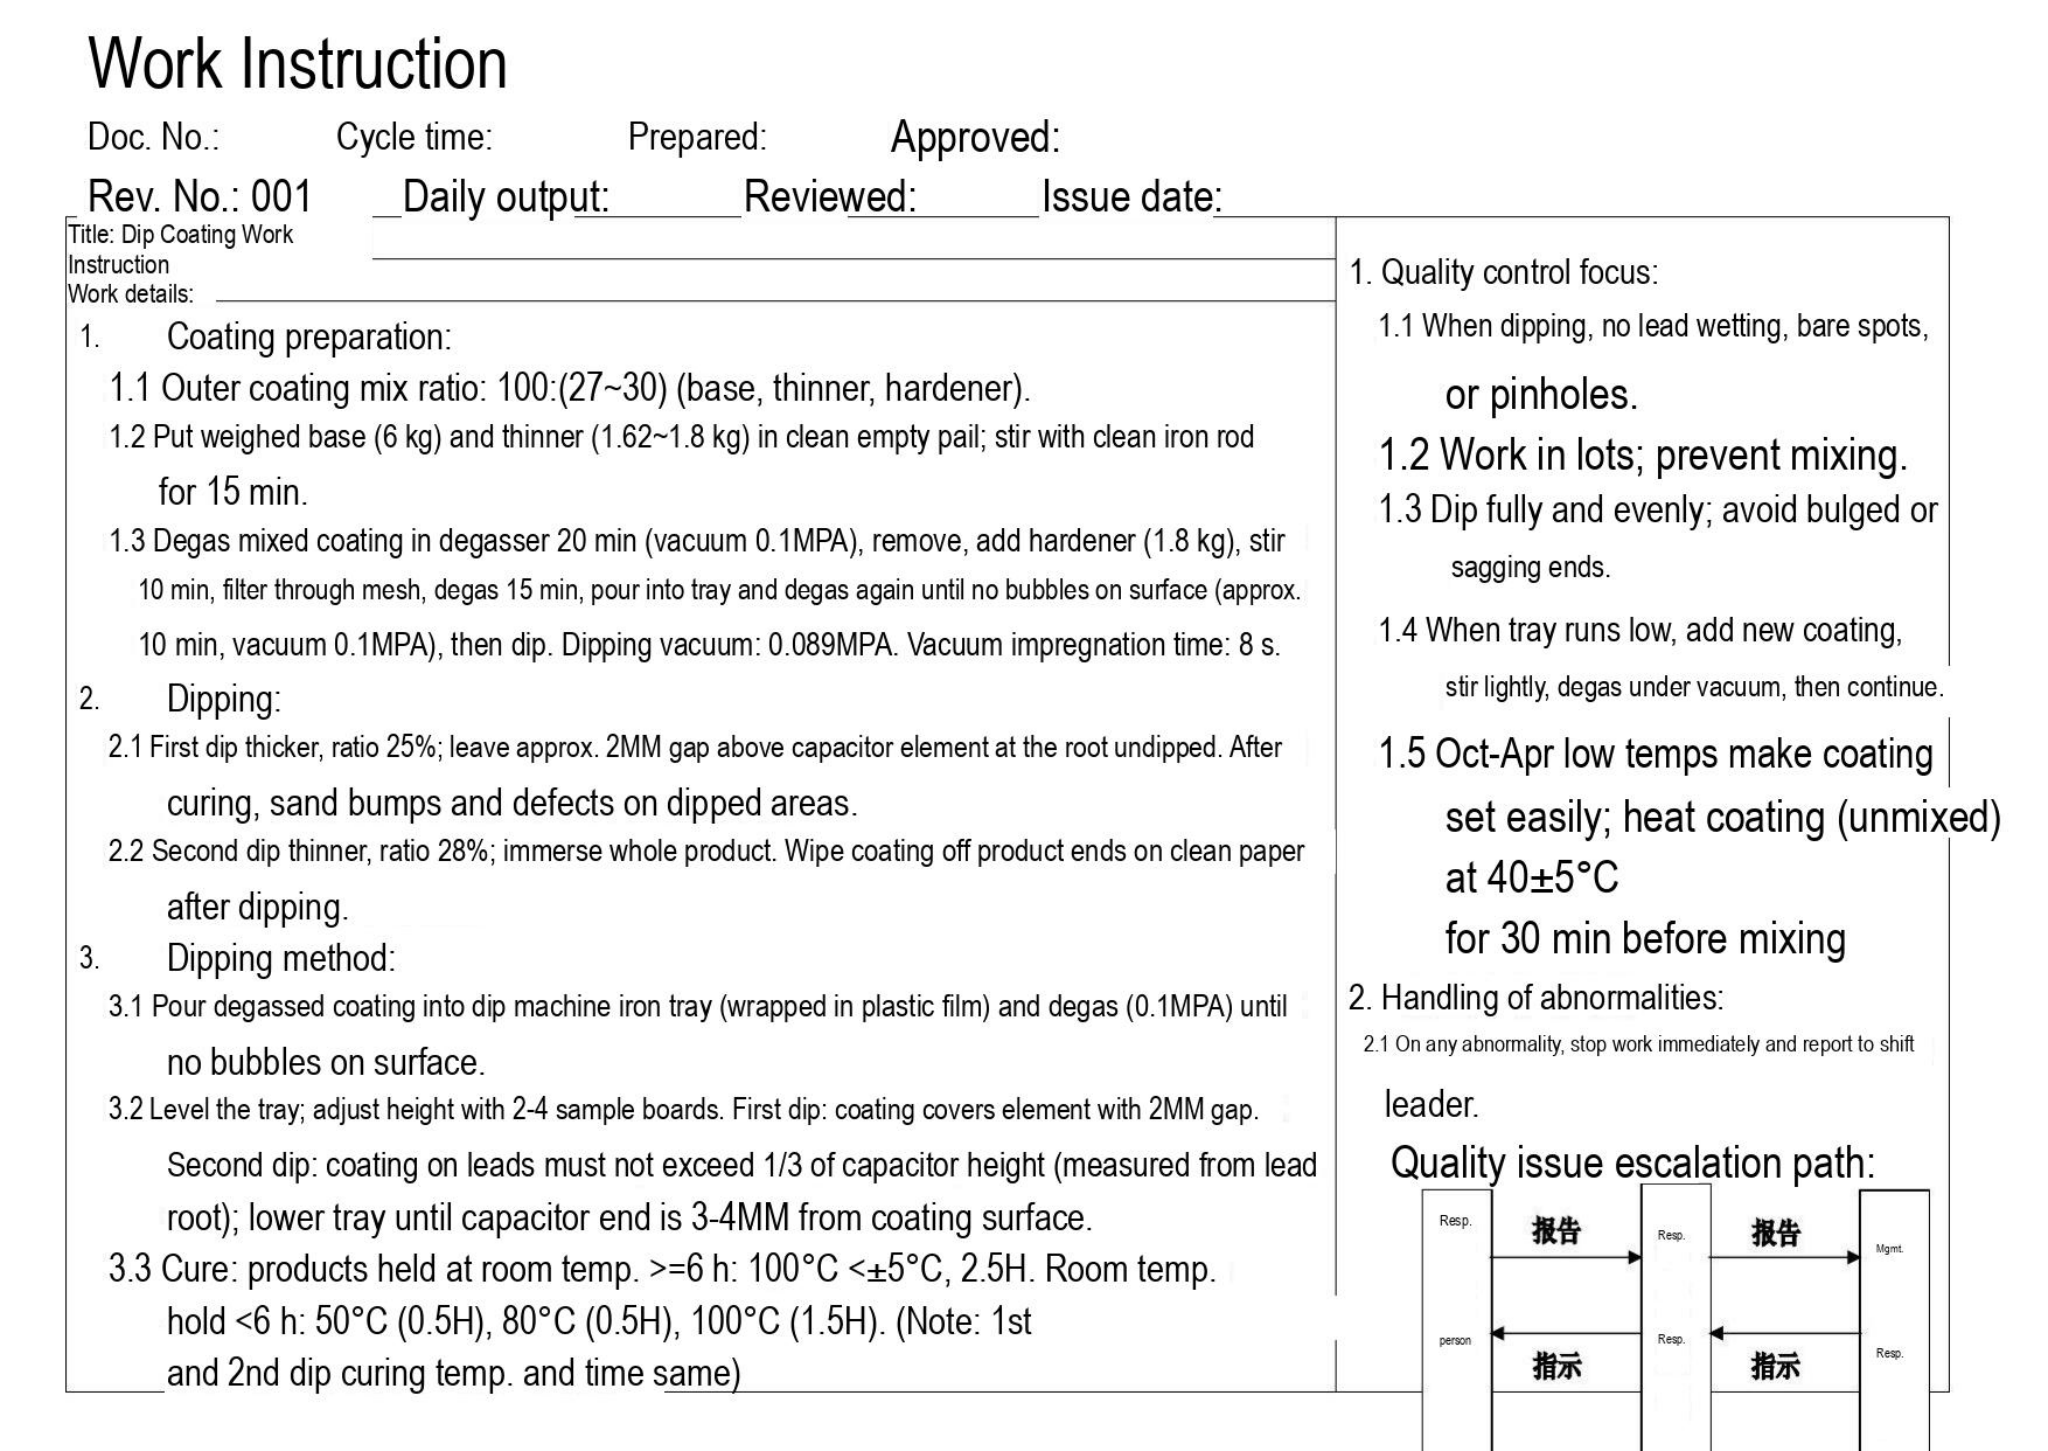# Work Instruction

Doc. No.: Cycle time: Prepared: Approved:

Rev. No.: 001 Daily output: Reviewed: Issue date:

Title: Dip Coating Work Instruction

Work details:

1. Coating preparation:

1.1 Outer coating mix ratio: 100:(27~30) (base, thinner, hardener).

1.2 Put weighed base (6 kg) and thinner (1.62~1.8 kg) in clean empty pail; stir with clean iron rod for 15 min.

1.3 Degas mixed coating in degasser 20 min (vacuum 0.1MPA), remove, add hardener (1.8 kg), stir 10 min, filter through mesh, degas 15 min, pour into tray and degas again until no bubbles on surface (approx. 10 min, vacuum 0.1MPA), then dip. Dipping vacuum: 0.089MPA. Vacuum impregnation time: 8 s.

2. Dipping:

2.1 First dip thicker, ratio 25%; leave approx. 2MM gap above capacitor element at the root undipped. After curing, sand bumps and defects on dipped areas.

2.2 Second dip thinner, ratio 28%; immerse whole product. Wipe coating off product ends on clean paper after dipping.

3. Dipping method:

3.1 Pour degassed coating into dip machine iron tray (wrapped in plastic film) and degas (0.1MPA) until no bubbles on surface.

3.2 Level the tray; adjust height with 2-4 sample boards. First dip: coating covers element with 2MM gap. Second dip: coating on leads must not exceed 1/3 of capacitor height (measured from lead root); lower tray until capacitor end is 3-4MM from coating surface.

3.3 Cure: products held at room temp. >=6 h: 100°C <±5°C, 2.5H. Room temp. hold <6 h: 50°C (0.5H), 80°C (0.5H), 100°C (1.5H). (Note: 1st and 2nd dip curing temp. and time same)

1. Quality control focus:

1.1 When dipping, no lead wetting, bare spots, or pinholes.

1.2 Work in lots; prevent mixing.

1.3 Dip fully and evenly; avoid bulged or sagging ends.

1.4 When tray runs low, add new coating, stir lightly, degas under vacuum, then continue.

1.5 Oct-Apr low temps make coating set easily; heat coating (unmixed) at 40±5°C for 30 min before mixing

2. Handling of abnormalities:

2.1 On any abnormality, stop work immediately and report to shift leader.

Quality issue escalation path:

Resp. 报告 Resp. 报告 Mgmt.

person 指示 Resp. 指示 Resp.
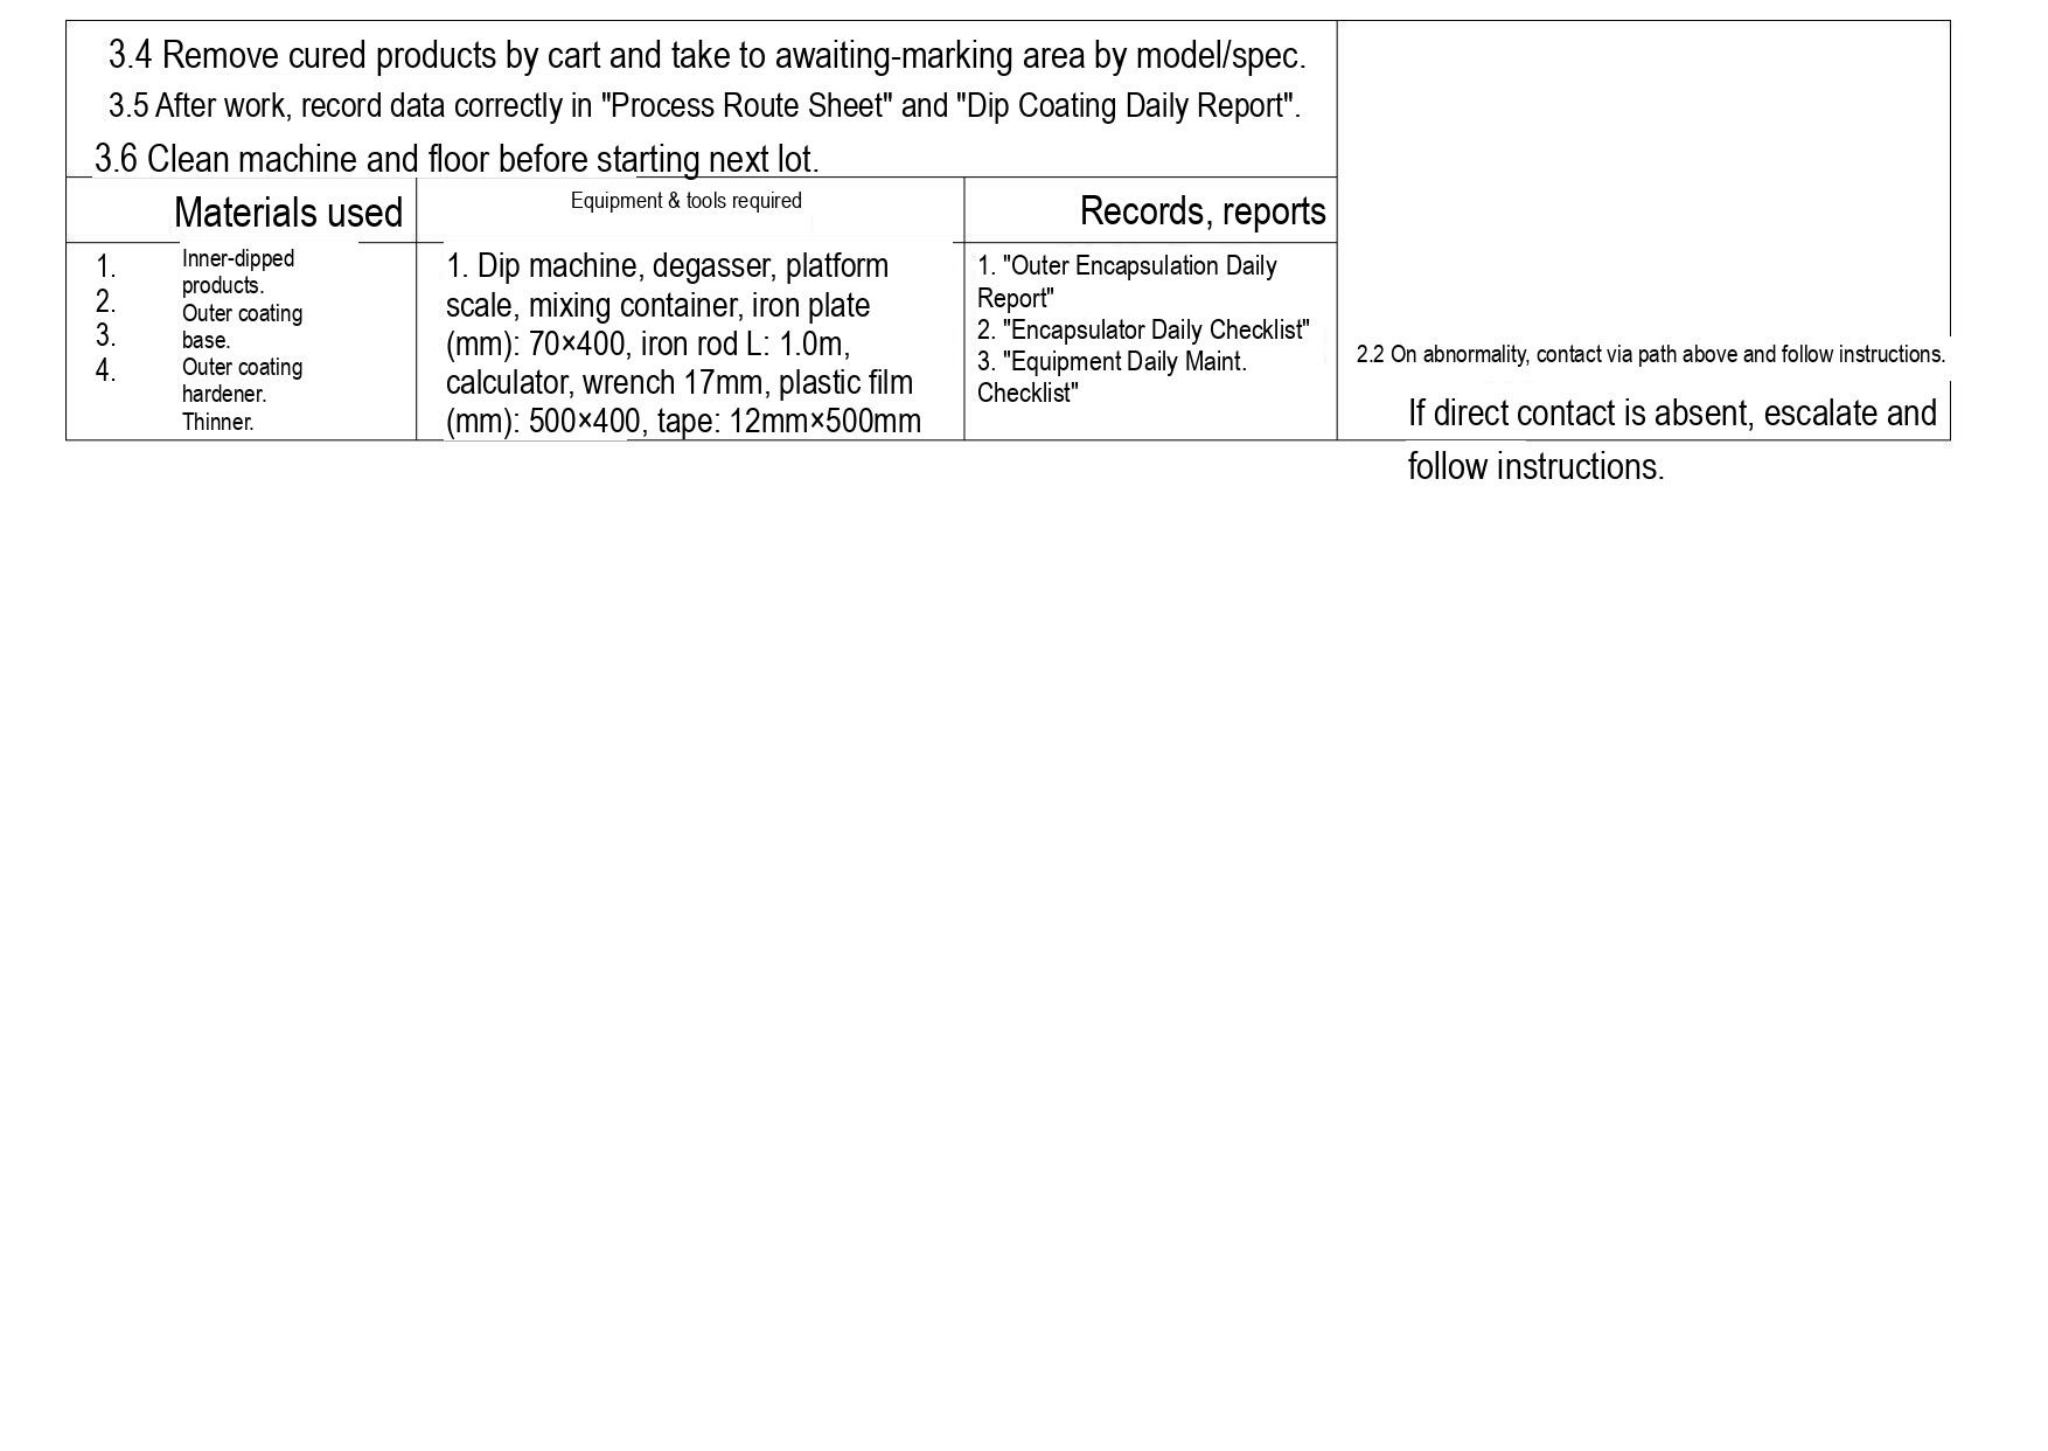3.4 Remove cured products by cart and take to awaiting-marking area by model/spec.
3.5 After work, record data correctly in "Process Route Sheet" and "Dip Coating Daily Report".
3.6 Clean machine and floor before starting next lot.

| Materials used | Equipment & tools required | Records, reports |
|---|---|---|
| 1. Inner-dipped products.<br>2. Outer coating base.<br>3. Outer coating hardener.<br>4. Thinner. | 1. Dip machine, degasser, platform scale, mixing container, iron plate (mm): 70×400, iron rod L: 1.0m, calculator, wrench 17mm, plastic film (mm): 500×400, tape: 12mm×500mm | 1. "Outer Encapsulation Daily Report"<br>2. "Encapsulator Daily Checklist"<br>3. "Equipment Daily Maint. Checklist" |

2.2 On abnormality, contact via path above and follow instructions.
If direct contact is absent, escalate and follow instructions.